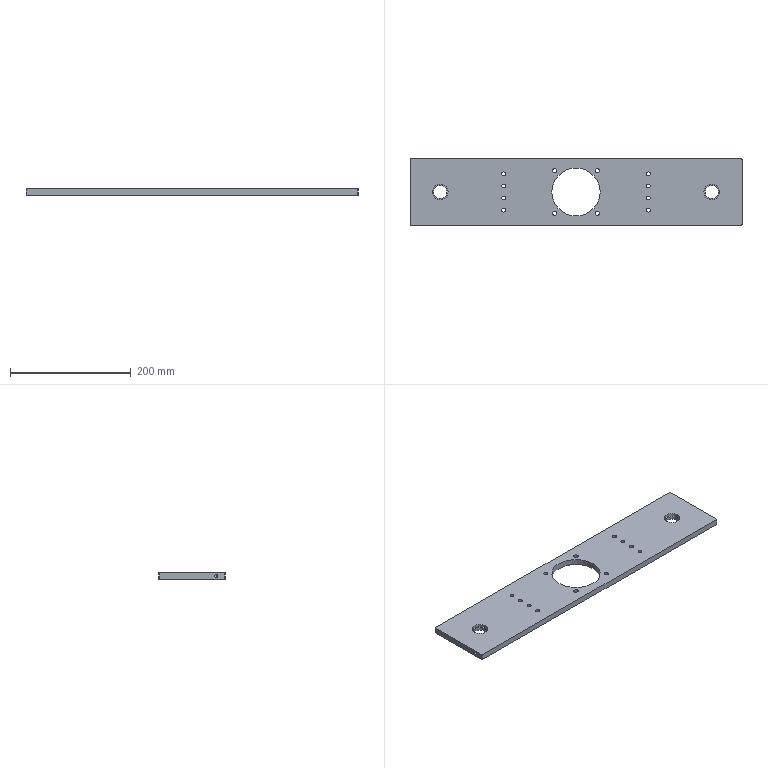Part | SolidWorks | features ICE 5, Extrusion 1, Fillet 1, HoleWzd 1, MirrorPattern 1 | 1 solid | 54 faces | box 550 x 110 x 10 mm | volume 540695 mm3 | cylinder 42 | plane 8 | cone 4 | commonest cylinder face diameters 6.5 x16 7 x8 2 x4 5 x4 22 x4 26 x4